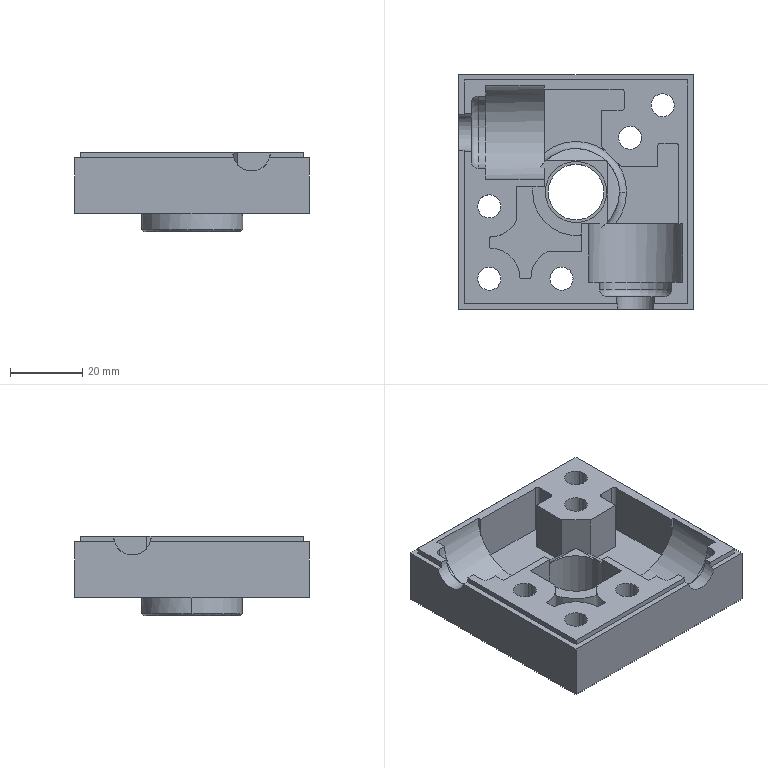Part | STEP file | Gear Box.1(Upper).stp | 1 solid | 101 faces | box 65 x 65 x 22 mm | volume 40348 mm3 | plane 51 | cylinder 44 | torus 4 | cone 2 | commonest cylinder face diameters 6.4 x10 11 x10 17 x5 2 x4 24 x3 10.4 x2